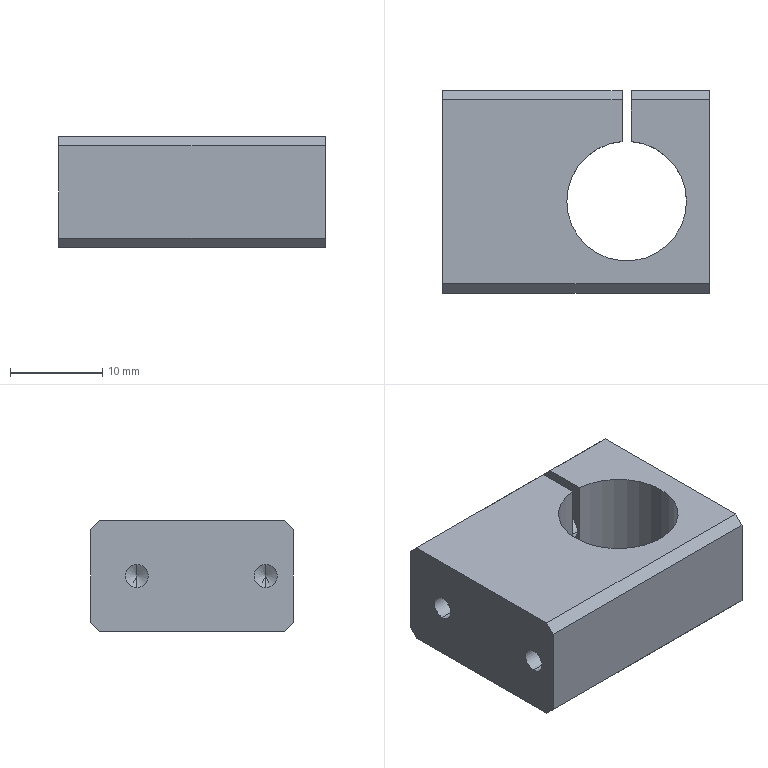NC program | NX | posted with a generic post | part box 29 x 22 x 12 mm
Whole program:
N10 G17 G21 G94 G90
(DRILLING_COPY_1_COPY_1 , TOOL : D6A45)
N12 T01 M6
N14 G54
N16 G17 G0 G90 X-6. Y0. B0. C0. S5000 M3
N18 G43 Z30. H1
N20 G94 G81 G98 Z-1.6 F250. R3.
N22 X8.
N24 G80
N26 G0 X8. Y0. Z30.
N28 M5
(DRILLING_COPY_1_COPY_COPY_COPY , TOOL : 2.5ZT)
N30 T12 M6
N32 G54
N34 G17 G0 G90 X-6. Y0. B0. C0. S2000 M3
N36 G43 Z30. H12
N38 G94 G83 G98 Z-18.251 F150. Q2. R3.
N40 X8.
N42 G80
N44 G0 X8. Y0. Z30.
N46 M5
(CUTTERCOMP11_COPY , TOOL : 2.3XYD)
N48 T11 M6
N50 G54
N52 G17 G0 G90 X-6. Y0. B0. C0. S5000 M3
N54 G43 Z30. H11
N56 Z1.564
N58 G42 G94 G1 X-6.078 Y-0.062 F850. D11
N60 X-6.128 Y-0.08 Z1.543
N62 X-6.175 Y-0.052 Z1.521
N64 X-6.183 Y0. Z1.5
N66 G2 X-6.183 Y0. Z1. I0.183 J0.
N68 X-6.183 Y0. Z0.5 I0.183 J0.
N70 X-6.183 Y0. Z0. I0.183 J0.
N72 X-6.183 Y0. Z-0.5 I0.183 J0.
N74 X-6.183 Y0. Z-1. I0.183 J0.
N76 X-6.183 Y0. Z-1.5 I0.183 J0.
N78 X-6.183 Y0. Z-2. I0.183 J0.
N80 X-6.183 Y0. Z-2.5 I0.183 J0.
N82 X-6.183 Y0. Z-3. I0.183 J0.
N84 X-6.183 Y0. Z-3.5 I0.183 J0.
N86 X-6.183 Y0. Z-4. I0.183 J0.
N88 X-6.183 Y0. Z-4.5 I0.183 J0.
N90 X-6.183 Y0. Z-5. I0.183 J0.
N92 X-6.183 Y0. Z-5.5 I0.183 J0.
N94 X-6.183 Y0. Z-6. I0.183 J0.
N96 X-6.183 Y0. Z-6.5 I0.183 J0.
N98 X-6.183 Y0. Z-7. I0.183 J0.
N100 X-6.183 Y0. Z-7.5 I0.183 J0.
N102 G1 X-6.175 Y0.052 Z-7.521
N104 X-6.128 Y0.08 Z-7.543
N106 X-6.078 Y0.062 Z-7.564
N108 G40
N110 X-6. Y0.
N112 G0 Z30.
N114 Z1.587
N116 G42 G1 X-6.055 Y-0.084
N118 G2 X-6.267 Y0. Z1.5 R0.123
N120 X-6.267 Y0. Z1. I0.267 J0.
N122 X-6.267 Y0. Z0.5 I0.267 J0.
N124 X-6.267 Y0. Z0. I0.267 J0.
N126 X-6.267 Y0. Z-0.5 I0.267 J0.
N128 X-6.267 Y0. Z-1. I0.267 J0.
N130 X-6.267 Y0. Z-1.5 I0.267 J0.
N132 X-6.267 Y0. Z-2. I0.267 J0.
N134 X-6.267 Y0. Z-2.5 I0.267 J0.
N136 X-6.267 Y0. Z-3. I0.267 J0.
N138 X-6.267 Y0. Z-3.5 I0.267 J0.
N140 X-6.267 Y0. Z-4. I0.267 J0.
N142 X-6.267 Y0. Z-4.5 I0.267 J0.
N144 X-6.267 Y0. Z-5. I0.267 J0.
N146 X-6.267 Y0. Z-5.5 I0.267 J0.
N148 X-6.267 Y0. Z-6. I0.267 J0.
N150 X-6.267 Y0. Z-6.5 I0.267 J0.
N152 X-6.267 Y0. Z-7. I0.267 J0.
N154 X-6.267 Y0. Z-7.5 I0.267 J0.
N156 X-6.055 Y0.084 Z-7.587 R0.123
N158 G40
N160 G1 X-6. Y0.
N162 G0 Z30.
N164 Z1.599
N166 G42 G1 X-6.039 Y-0.092
N168 G2 X-6.35 Y0. Z1.5 R0.169
N170 X-6.35 Y0. Z1. I0.35 J0.
N172 X-6.35 Y0. Z0.5 I0.35 J0.
N174 X-6.35 Y0. Z0. I0.35 J0.
N176 X-6.35 Y0. Z-0.5 I0.35 J0.
N178 X-6.35 Y0. Z-1. I0.35 J0.
N180 X-6.35 Y0. Z-1.5 I0.35 J0.
N182 X-6.35 Y0. Z-2. I0.35 J0.
N184 X-6.35 Y0. Z-2.5 I0.35 J0.
N186 X-6.35 Y0. Z-3. I0.35 J0.
N188 X-6.35 Y0. Z-3.5 I0.35 J0.
N190 X-6.35 Y0. Z-4. I0.35 J0.
N192 X-6.35 Y0. Z-4.5 I0.35 J0.
N194 X-6.35 Y0. Z-5. I0.35 J0.
N196 X-6.35 Y0. Z-5.5 I0.35 J0.
N198 X-6.35 Y0. Z-6. I0.35 J0.
N200 X-6.35 Y0. Z-6.5 I0.35 J0.
N202 X-6.35 Y0. Z-7. I0.35 J0.
N204 X-6.35 Y0. Z-7.5 I0.35 J0.
N206 X-6.039 Y0.092 Z-7.599 R0.169
N208 G40
N210 G1 X-6. Y0.
N212 G0 Z30.
N214 X8.
N216 Z1.564
N218 G42 G1 X7.922 Y-0.062
N220 X7.872 Y-0.08 Z1.543
N222 X7.825 Y-0.052 Z1.521
N224 X7.817 Y0. Z1.5
N226 G2 X7.817 Y0. Z1. I0.183 J0.
N228 X7.817 Y0. Z0.5 I0.183 J0.
N230 X7.817 Y0. Z0. I0.183 J0.
N232 X7.817 Y0. Z-0.5 I0.183 J0.
N234 X7.817 Y0. Z-1. I0.183 J0.
N236 X7.817 Y0. Z-1.5 I0.183 J0.
N238 X7.817 Y0. Z-2. I0.183 J0.
N240 X7.817 Y0. Z-2.5 I0.183 J0.
N242 X7.817 Y0. Z-3. I0.183 J0.
N244 X7.817 Y0. Z-3.5 I0.183 J0.
N246 X7.817 Y0. Z-4. I0.183 J0.
N248 X7.817 Y0. Z-4.5 I0.183 J0.
N250 X7.817 Y0. Z-5. I0.183 J0.
N252 X7.817 Y0. Z-5.5 I0.183 J0.
N254 X7.817 Y0. Z-6. I0.183 J0.
N256 X7.817 Y0. Z-6.5 I0.183 J0.
N258 X7.817 Y0. Z-7. I0.183 J0.
N260 X7.817 Y0. Z-7.5 I0.183 J0.
N262 G1 X7.825 Y0.052 Z-7.521
N264 X7.872 Y0.08 Z-7.543
N266 X7.922 Y0.062 Z-7.564
N268 G40
N270 X8. Y0.
N272 G0 Z30.
N274 Z1.587
N276 G42 G1 X7.945 Y-0.084
N278 G2 X7.733 Y0. Z1.5 R0.123
N280 X7.733 Y0. Z1. I0.267 J0.
N282 X7.733 Y0. Z0.5 I0.267 J0.
N284 X7.733 Y0. Z0. I0.267 J0.
N286 X7.733 Y0. Z-0.5 I0.267 J0.
N288 X7.733 Y0. Z-1. I0.267 J0.
N290 X7.733 Y0. Z-1.5 I0.267 J0.
N292 X7.733 Y0. Z-2. I0.267 J0.
N294 X7.733 Y0. Z-2.5 I0.267 J0.
N296 X7.733 Y0. Z-3. I0.267 J0.
N298 X7.733 Y0. Z-3.5 I0.267 J0.
N300 X7.733 Y0. Z-4. I0.267 J0.
N302 X7.733 Y0. Z-4.5 I0.267 J0.
N304 X7.733 Y0. Z-5. I0.267 J0.
N306 X7.733 Y0. Z-5.5 I0.267 J0.
N308 X7.733 Y0. Z-6. I0.267 J0.
N310 X7.733 Y0. Z-6.5 I0.267 J0.
N312 X7.733 Y0. Z-7. I0.267 J0.
N314 X7.733 Y0. Z-7.5 I0.267 J0.
N316 X7.945 Y0.084 Z-7.587 R0.123
N318 G40
N320 G1 X8. Y0.
N322 G0 Z30.
N324 Z1.599
N326 G42 G1 X7.961 Y-0.092
N328 G2 X7.65 Y0. Z1.5 R0.169
N330 X7.65 Y0. Z1. I0.35 J0.
N332 X7.65 Y0. Z0.5 I0.35 J0.
N334 X7.65 Y0. Z0. I0.35 J0.
N336 X7.65 Y0. Z-0.5 I0.35 J0.
N338 X7.65 Y0. Z-1. I0.35 J0.
N340 X7.65 Y0. Z-1.5 I0.35 J0.
N342 X7.65 Y0. Z-2. I0.35 J0.
N344 X7.65 Y0. Z-2.5 I0.35 J0.
N346 X7.65 Y0. Z-3. I0.35 J0.
N348 X7.65 Y0. Z-3.5 I0.35 J0.
N350 X7.65 Y0. Z-4. I0.35 J0.
N352 X7.65 Y0. Z-4.5 I0.35 J0.
N354 X7.65 Y0. Z-5. I0.35 J0.
N356 X7.65 Y0. Z-5.5 I0.35 J0.
N358 X7.65 Y0. Z-6. I0.35 J0.
N360 X7.65 Y0. Z-6.5 I0.35 J0.
N362 X7.65 Y0. Z-7. I0.35 J0.
N364 X7.65 Y0. Z-7.5 I0.35 J0.
N366 X7.961 Y0.092 Z-7.599 R0.169
N368 G40
N370 G1 X8. Y0.
N372 G0 Z30.
N374 M5
N376 M2